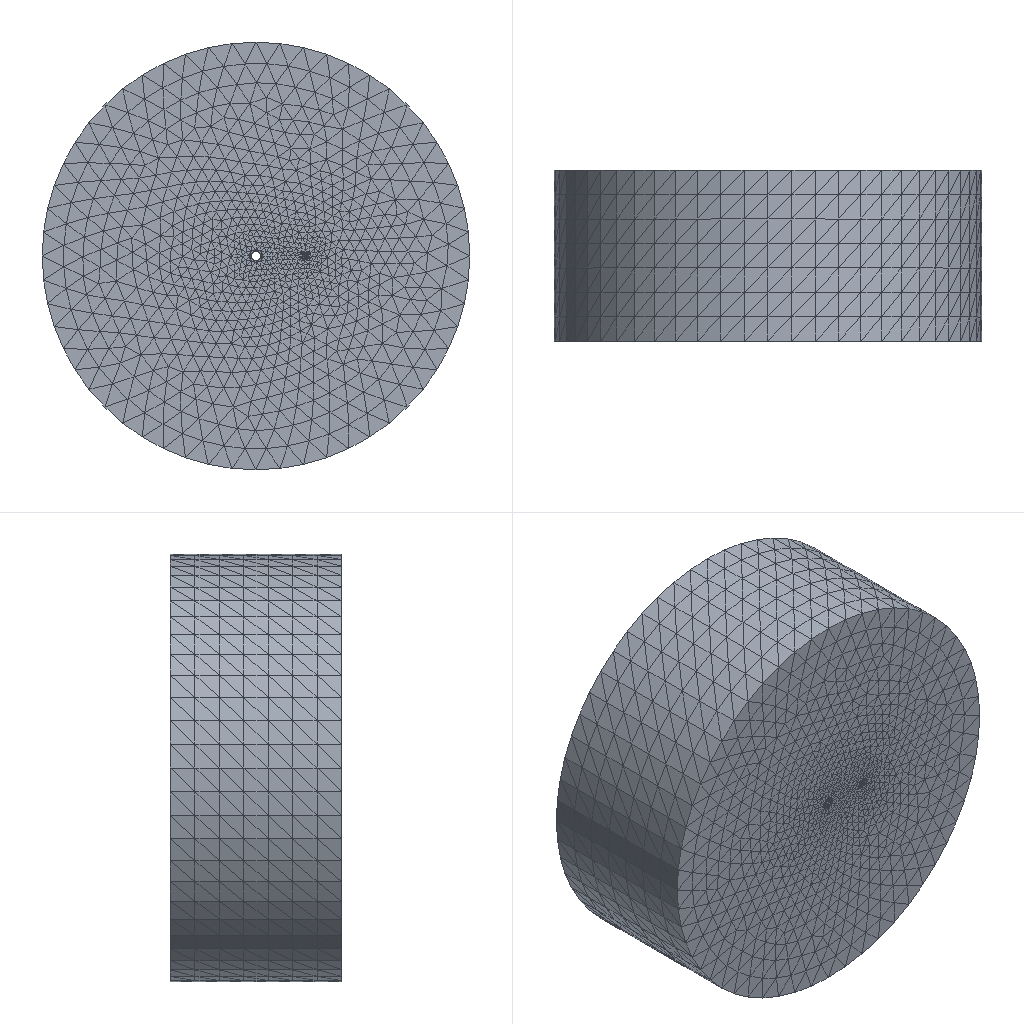Simulation study | abaqus
Set-up summary:
category,name,step,type,value,unit,region
solver,abaqus
solver,version,,,Abaqus/Standard 2020
units,not stated in the deck,,not stated
analysis,deck,,static,static
load_step,Step-1,Step-1,static
load_step,Step-2,Step-2,static
load_step,requested,,,2
mesh,nodes,,,19342
mesh,elements,,,80560
element_type,C3D4,,solid,80560
load,load commands in deck,,count,1
bc,support commands in deck,,count,1
material,CEMENT,,in results
material,SOIL,,in results
material,TUBE,,in results
check,setup vs results,,match,"per instance, exact: element labels, types and connectivity; labels of the nodes the elements use; coordinates of those nodes at SINGLE_PRECISION in 1 of 3 instance(s)"
Abaqus input file, long lists of numbers shortened:
*Heading
** Job name: Job-2 Model name: Model-1-Copy
** Generated by: Abaqus/CAE 2020
*Preprint, echo=NO, model=NO, history=NO, contact=NO
**
** PARTS
**
*Part, name=P21
*Node
      1,   1050.777,           0.,           0.
      2,   1258.624,           0.,           0.
** (8455 more lines like these left out)
*Element, type=C3D4
    1, 7574, 7583, 3286, 7573
    2, 7581, 3288, 3287, 3349
** (25295 more lines like these left out)
*Nset, nset=Set-1, generate
    1,  8457,     1
*Elset, elset=Set-1, generate
     1,  25297,      1
** Section: tube
*Solid Section, elset=Set-1, material=tube
,
*End Part
**
*Part, name=P22
*Node
      1,   1012.672,           0.,           0.
      2,   1296.729,           0.,           0.
** (1206 more lines like these left out)
*Element, type=C3D4
   1, 1188, 1190,  609, 1193
   2, 1188,    8, 1191,  610
** (3563 more lines like these left out)
*Nset, nset=Set-1, generate
    1,  1208,     1
*Elset, elset=Set-1, generate
    1,  3565,     1
*Nset, nset=Set-2, generate
    1,  1208,     1
*Elset, elset=Set-2, generate
    1,  3565,     1
** Section: cement
*Solid Section, elset=Set-2, material=cement
,
*End Part
**
*Part, name=P23
*Node
      1,           0.,           0.,        5000.
      2,           0.,           0.,       -5000.
** (9675 more lines like these left out)
*Element, type=C3D4
    1, 2201, 2202, 2203, 2204
    2, 2201, 2202, 2205, 2203
** (51696 more lines like these left out)
*Nset, nset=Set-1, generate
    1,  9677,     1
*Elset, elset=Set-1, generate
     1,  51698,      1
** Section: soil
*Solid Section, elset=Set-1, material=soil
,
*End Part
**
**
** ASSEMBLY
**
*Assembly, name=Assembly
**
*Instance, name=P21-1, part=P21
*End Instance
**
*Instance, name=P22-1, part=P22
*End Instance
**
*Instance, name=P23-1, part=P23
          0.,        4000.,           0.
          0.,        4000.,           0.,           1.,        4000., 6.12323426292584e-17,         180.
*End Instance
**
*Nset, nset=Set-1, instance=P21-1
   1,   2,   3,   4,   9,  10,  11,  12,  17,  18,  19,  20,  21,  22,  23,  24
  25,  26,  27,  28,  29,  30,  31,  32,  33,  34,  35,  36,  37,  38,  39,  40
** (4 more lines like these left out)
*Nset, nset=Set-1, instance=P22-1
   1,   2,   3,   4,   9,  10,  11,  12,  17,  18,  19,  20,  21,  22,  23,  24
  25,  26,  27,  28, 102, 103, 104, 105, 106, 107, 108, 109, 110, 111, 112, 113
** (1 more lines like these left out)
*Nset, nset=Set-1, instance=P23-1
    5,    6,    9,   10,   11,   12,   88,   89,   90,   91,   92,   93,  112,  113,  114,  115
  116,  117,  124,  125,  126,  127,  128,  129,  130,  131,  132,  133,  134,  135,  136,  137
** (53 more lines like these left out)
*Elset, elset=Set-1, instance=P21-1
   838,   844,   850,   902,   938,  1491,  6031, 10297, 10301, 10312, 10314, 10326, 10328, 10341, 10342, 10361
 10389, 10392, 10394, 10405, 10420, 10436, 10440, 10451, 10465, 10466, 10468, 10473, 10474, 10481, 10482, 10487
** (4 more lines like these left out)
*Elset, elset=Set-1, instance=P22-1
  149,  506, 1424, 1821, 1826, 1873, 1874, 1875, 1877, 1884, 1888, 1903, 1908, 1922, 1933, 1938
 1939, 1941, 2226, 2269, 2361, 2533, 2537, 2561, 2767, 2825, 2836, 2842, 2846, 2847, 2848, 3042
** (1 more lines like these left out)
*Elset, elset=Set-1, instance=P23-1
    15,   152,   213,   350,   508,   532,   550,   619,   665,   831,  1279,  1311,  1422,  1458,  1522,  1597
  1651,  1745,  1796,  1807,  1938,  2013,  2113,  2181,  2314,  2352,  2353,  2435,  2530,  2604,  2626,  2627
** (103 more lines like these left out)
*Nset, nset=Set-2, instance=P21-1, generate
    1,  8457,     1
*Nset, nset=Set-2, instance=P22-1, generate
    1,  1208,     1
*Nset, nset=Set-2, instance=P23-1, generate
    1,  9677,     1
*Elset, elset=Set-2, instance=P21-1, generate
     1,  25297,      1
*Elset, elset=Set-2, instance=P22-1, generate
    1,  3565,     1
*Elset, elset=Set-2, instance=P23-1, generate
     1,  51698,      1
*Nset, nset=Set-3, instance=P21-1, generate
    1,  8457,     1
*Nset, nset=Set-3, instance=P22-1, generate
    1,  1208,     1
*Nset, nset=Set-3, instance=P23-1, generate
    1,  9677,     1
*Elset, elset=Set-3, instance=P21-1, generate
     1,  25297,      1
*Elset, elset=Set-3, instance=P22-1, generate
    1,  3565,     1
*Elset, elset=Set-3, instance=P23-1, generate
     1,  51698,      1
*Nset, nset=Set-4, instance=P21-1, generate
    1,  8457,     1
*Nset, nset=Set-4, instance=P22-1, generate
    1,  1208,     1
*Nset, nset=Set-4, instance=P23-1, generate
    1,  9677,     1
*Elset, elset=Set-4, instance=P21-1, generate
     1,  25297,      1
*Elset, elset=Set-4, instance=P22-1, generate
    1,  3565,     1
*Elset, elset=Set-4, instance=P23-1, generate
     1,  51698,      1
*Elset, elset=_Surf-1_S3, internal, instance=P21-1
     2,     3,     8,    15,    31,    34,    47,    52,    72,    76,    84,    95,    96,   102,   110,   123
   124,   147,   149,   153,   177,   183,   185,   186,   189,   202,   206,   207,   217,   228,   235,   245
** (439 more lines like these left out)
*Elset, elset=_Surf-1_S4, internal, instance=P21-1
    29,    37,   119,   143,   154,   167,   325,   397,   465,   499,   565,   610,   652,   667,   673,   718
   773,   838,   844,   864,   913,   920,   938,   945,   955,   966,   992,  1009,  1011,  1015,  1066,  1087
** (22 more lines like these left out)
*Elset, elset=_Surf-1_S1, internal, instance=P21-1
   223,   420,   443,   459,   693,   785,   830,   866,  1608,  1623,  2301,  2526,  3215,  3218,  3593,  3598
  3692,  4192,  4402,  4443,  4547,  4582,  4586,  4798,  5314,  5372,  5657,  5929,  6073,  6639,  6643,  7053
** (13 more lines like these left out)
*Elset, elset=_Surf-1_S2, internal, instance=P21-1
    21,    54,   273,   331,   336,   367,   449,   491,   522,   543,   612,   653,   655,   658,  1065,  1111
  1139,  1180,  1261,  1290,  1705,  2255,  2774,  2778,  2863,  3034,  3327,  3662,  4244,  4304,  4344,  4485
** (16 more lines like these left out)
*Surface, type=ELEMENT, name=Surf-1
_Surf-1_S3, S3
_Surf-1_S4, S4
_Surf-1_S2, S2
_Surf-1_S1, S1
*Elset, elset=_Surf-2_S4, internal, instance=P21-1
    11,    13,    26,    29,    37,    38,    58,    59,    78,    88,    93,   112,   119,   122,   127,   143
   145,   154,   159,   167,   171,   174,   187,   190,   196,   199,   212,   243,   262,   285,   297,   300
** (158 more lines like these left out)
*Elset, elset=_Surf-2_S4, internal, instance=P22-1
    7,   12,   22,   26,   32,   54,   55,   59,   61,   75,   87,  104,  106,  125,  141,  142
  169,  170,  182,  189,  192,  194,  199,  203,  219,  226,  235,  241,  243,  258,  259,  288
** (23 more lines like these left out)
*Elset, elset=_Surf-2_S4, internal, instance=P23-1
   293,  1215,  1422,  1704,  2620,  2635,  2721,  2737,  2758,  2882,  2966,  3146,  3160,  3288,  3450,  3914
  4023,  4055,  4489,  4644,  4717,  4811,  4903,  5114,  5203,  5349,  5376,  5379,  5392,  5576,  5614,  5738
** (8 more lines like these left out)
*Elset, elset=_Surf-2_S2, internal, instance=P21-1
     1,     7,    12,    21,    23,    27,    35,    54,    56,    66,    67,    74,    77,    90,    94,    99
   105,   116,   125,   131,   134,   135,   140,   144,   156,   160,   161,   168,   178,   181,   184,   191
** (204 more lines like these left out)
*Elset, elset=_Surf-2_S2, internal, instance=P22-1
    1,    3,   14,   18,   23,   25,   36,   38,   39,   41,   45,   56,   66,   71,   73,   78
   79,   84,   90,   92,   93,   99,  100,  101,  107,  116,  117,  121,  122,  126,  129,  136
** (35 more lines like these left out)
*Elset, elset=_Surf-2_S2, internal, instance=P23-1
    15,   213,  1425,  2671,  2680,  2681,  2697,  2946,  3058,  3136,  3248,  3276,  3288,  3625,  3774,  3778
  3922,  4321,  4378,  4380,  4426,  4580,  4736,  4740,  4848,  4913,  5018,  5098,  5140,  5172,  5368,  5369
** (10 more lines like these left out)
*Elset, elset=_Surf-2_S1, internal, instance=P21-1
    17,    18,    19,    28,    42,    45,    46,    48,    57,    63,    71,    73,    79,    80,    82,    89
   100,   104,   111,   113,   117,   120,   136,   137,   150,   169,   173,   188,   193,   194,   197,   201
** (219 more lines like these left out)
*Elset, elset=_Surf-2_S1, internal, instance=P22-1
    2,    4,    6,    8,   10,   15,   16,   20,   21,   27,   28,   37,   43,   44,   51,   53
   63,   64,   69,   80,   86,   94,  102,  111,  130,  133,  148,  149,  156,  157,  162,  167
** (28 more lines like these left out)
*Elset, elset=_Surf-2_S1, internal, instance=P23-1
  2647,  2650,  2681,  2737,  4903,  5051,  5114,  5379,  5562,  5942,  5948,  5991,  6048,  6147,  6285,  6327
  6728,  6913,  7548,  7761,  7950,  7962,  8070,  8084,  8120,  8147,  8159,  8448,  8627,  8801,  8819,  8866
** (6 more lines like these left out)
*Elset, elset=_Surf-2_S3, internal, instance=P21-1
     2,     3,     8,    15,    31,    34,    47,    52,    72,    76,    84,    85,    95,    96,   102,   106
   108,   110,   123,   124,   141,   147,   149,   153,   175,   177,   183,   185,   186,   189,   202,   206
** (467 more lines like these left out)
*Elset, elset=_Surf-2_S3, internal, instance=P22-1
   13,   17,   24,   35,   47,   50,   97,   98,  108,  110,  113,  114,  115,  118,  128,  134
  137,  139,  144,  151,  153,  160,  161,  163,  174,  176,  196,  201,  207,  209,  212,  214
** (59 more lines like these left out)
*Elset, elset=_Surf-2_S3, internal, instance=P23-1
    27,    30,    53,    61,    90,   113,   114,   152,   174,   210,   218,   350,   398,   498,   502,   503
   508,   532,   550,   619,   665,   741,   831,   847,   928,  1058,  1143,  1209,  1243,  1279,  1311,  1319
** (245 more lines like these left out)
*Surface, type=ELEMENT, name=Surf-2
_Surf-2_S4, S4
_Surf-2_S2, S2
_Surf-2_S1, S1
_Surf-2_S3, S3
*Elset, elset=_Surf-3_S4, internal, instance=P21-1
    11,    13,    26,    29,    37,    38,    58,    59,    78,    88,    93,   112,   119,   122,   127,   143
   145,   154,   159,   167,   171,   174,   187,   190,   196,   199,   212,   243,   262,   285,   297,   300
** (158 more lines like these left out)
*Elset, elset=_Surf-3_S4, internal, instance=P22-1
    7,   12,   22,   26,   32,   54,   55,   59,   61,   75,   87,  104,  106,  125,  141,  142
  169,  170,  182,  189,  192,  194,  199,  203,  219,  226,  235,  241,  243,  258,  259,  288
** (23 more lines like these left out)
*Elset, elset=_Surf-3_S4, internal, instance=P23-1
   293,  1215,  1422,  1704,  2620,  2635,  2721,  2737,  2758,  2882,  2966,  3146,  3160,  3288,  3450,  3914
  4023,  4055,  4489,  4644,  4717,  4811,  4903,  5114,  5203,  5349,  5376,  5379,  5392,  5576,  5614,  5738
** (8 more lines like these left out)
*Elset, elset=_Surf-3_S2, internal, instance=P21-1
     1,     7,    12,    21,    23,    27,    35,    54,    56,    66,    67,    74,    77,    90,    94,    99
   105,   116,   125,   131,   134,   135,   140,   144,   156,   160,   161,   168,   178,   181,   184,   191
** (204 more lines like these left out)
*Elset, elset=_Surf-3_S2, internal, instance=P22-1
    1,    3,   14,   18,   23,   25,   36,   38,   39,   41,   45,   56,   66,   71,   73,   78
   79,   84,   90,   92,   93,   99,  100,  101,  107,  116,  117,  121,  122,  126,  129,  136
** (35 more lines like these left out)
*Elset, elset=_Surf-3_S2, internal, instance=P23-1
    15,   213,  1425,  2671,  2680,  2681,  2697,  2946,  3058,  3136,  3248,  3276,  3288,  3625,  3774,  3778
  3922,  4321,  4378,  4380,  4426,  4580,  4736,  4740,  4848,  4913,  5018,  5098,  5140,  5172,  5368,  5369
** (10 more lines like these left out)
*Elset, elset=_Surf-3_S1, internal, instance=P21-1
    17,    18,    19,    28,    42,    45,    46,    48,    57,    63,    71,    73,    79,    80,    82,    89
   100,   104,   111,   113,   117,   120,   136,   137,   150,   169,   173,   188,   193,   194,   197,   201
** (219 more lines like these left out)
*Elset, elset=_Surf-3_S1, internal, instance=P22-1
    2,    4,    6,    8,   10,   15,   16,   20,   21,   27,   28,   37,   43,   44,   51,   53
   63,   64,   69,   80,   86,   94,  102,  111,  130,  133,  148,  149,  156,  157,  162,  167
** (28 more lines like these left out)
*Elset, elset=_Surf-3_S1, internal, instance=P23-1
  2647,  2650,  2681,  2737,  4903,  5051,  5114,  5379,  5562,  5942,  5948,  5991,  6048,  6147,  6285,  6327
  6728,  6913,  7548,  7761,  7950,  7962,  8070,  8084,  8120,  8147,  8159,  8448,  8627,  8801,  8819,  8866
** (6 more lines like these left out)
*Elset, elset=_Surf-3_S3, internal, instance=P21-1
     2,     3,     8,    15,    31,    34,    47,    52,    72,    76,    84,    85,    95,    96,   102,   106
   108,   110,   123,   124,   141,   147,   149,   153,   175,   177,   183,   185,   186,   189,   202,   206
** (467 more lines like these left out)
*Elset, elset=_Surf-3_S3, internal, instance=P22-1
   13,   17,   24,   35,   47,   50,   97,   98,  108,  110,  113,  114,  115,  118,  128,  134
  137,  139,  144,  151,  153,  160,  161,  163,  174,  176,  196,  201,  207,  209,  212,  214
** (59 more lines like these left out)
*Elset, elset=_Surf-3_S3, internal, instance=P23-1
    27,    30,    53,    61,    90,   113,   114,   152,   174,   210,   218,   350,   398,   498,   502,   503
   508,   532,   550,   619,   665,   741,   831,   847,   928,  1058,  1143,  1209,  1243,  1279,  1311,  1319
** (245 more lines like these left out)
*Surface, type=ELEMENT, name=Surf-3
_Surf-3_S4, S4
_Surf-3_S2, S2
_Surf-3_S1, S1
_Surf-3_S3, S3
*Elset, elset=_m_Surf-4_S2, internal, instance=P21-1
     1,     7,    12,    23,    27,    35,    56,    66,    67,    74,    77,    90,    94,    99,   105,   116
   125,   131,   134,   135,   140,   144,   156,   160,   161,   168,   178,   181,   184,   191,   215,   216
** (137 more lines like these left out)
*Elset, elset=_m_Surf-4_S4, internal, instance=P21-1
    11,    13,    26,    38,    58,    78,    88,    93,   112,   122,   127,   145,   159,   171,   174,   187
   190,   196,   199,   212,   243,   262,   285,   297,   300,   316,   337,   344,   352,   378,   390,   404
** (90 more lines like these left out)
*Elset, elset=_m_Surf-4_S1, internal, instance=P21-1
    17,    18,    19,    28,    42,    45,    46,    48,    57,    63,    71,    73,    79,    80,    82,    89
   100,   104,   111,   113,   117,   120,   136,   137,   150,   169,   173,   188,   193,   194,   197,   201
** (148 more lines like these left out)
*Elset, elset=_m_Surf-4_S3, internal, instance=P21-1
    85,   106,   108,   141,   175,   211,   272,   345,   348,   368,   376,   417,   462,   471,   492,   498
   550,   551,   554,   564,   615,   640,   661,   682,   687,   735,   765,   803,   811,   889,   901,   915
** (17 more lines like these left out)
*Surface, type=ELEMENT, name=m_Surf-4
_m_Surf-4_S2, S2
_m_Surf-4_S4, S4
_m_Surf-4_S1, S1
_m_Surf-4_S3, S3
*Elset, elset=_m_Surf-6_S2, internal, instance=P22-1
    1,    3,   14,   18,   23,   25,   36,   38,   39,   41,   45,   66,   71,   73,   78,   79
   90,   93,   99,  100,  101,  107,  116,  117,  121,  122,  129,  136,  140,  147,  158,  159
** (19 more lines like these left out)
*Elset, elset=_m_Surf-6_S1, internal, instance=P22-1
    2,    6,    8,   10,   15,   16,   21,   27,   28,   37,   43,   44,   51,   53,   63,   64
   80,   94,  102,  111,  130,  133,  156,  157,  162,  167,  172,  173,  181,  197,  198,  215
** (15 more lines like these left out)
*Elset, elset=_m_Surf-6_S4, internal, instance=P22-1
    7,   12,   22,   26,   32,   54,   55,  104,  141,  142,  169,  170,  182,  199,  203,  226
  241,  259,  288,  304,  322,  323,  331,  355,  359,  385,  418,  425,  436,  443,  455,  462
** (8 more lines like these left out)
*Elset, elset=_m_Surf-6_S3, internal, instance=P22-1
   17,   50,  108,  114,  118,  134,  151,  153,  161,  176,  196,  209,  255,  264,  271,  289
  310,  551,  611,  734,  789,  805,  816,  827,  844,  918,  939,  943,  956,  975, 1002, 1009
** (2 more lines like these left out)
*Surface, type=ELEMENT, name=m_Surf-6
_m_Surf-6_S2, S2
_m_Surf-6_S1, S1
_m_Surf-6_S4, S4
_m_Surf-6_S3, S3
*Elset, elset=_s_Surf-4_S2, internal, instance=P22-1
   56,   84,  126,  263,  277,  460,  613,  614,  699,  748,  752,  904, 1102, 1108, 1251, 1252
 1274, 1283, 1333, 1337, 1338, 1339, 1373, 1429, 1443, 1447, 1450, 1451, 1467, 1553, 1584, 1673
** (4 more lines like these left out)
*Elset, elset=_s_Surf-4_S3, internal, instance=P22-1
   13,   24,   35,   47,   97,   98,  110,  113,  115,  128,  137,  139,  144,  160,  163,  174
  201,  207,  212,  214,  223,  228,  231,  233,  234,  238,  245,  267,  273,  274,  278,  281
** (53 more lines like these left out)
*Elset, elset=_s_Surf-4_S1, internal, instance=P22-1
    4,   20,   69,   86,  148,  149,  175,  188,  266,  369,  440,  478,  536,  722,  741,  757
  764,  857,  885,  898,  902,  909,  919,  992, 1077, 1093, 1117, 1120, 1302, 1380, 1445, 1448
** (4 more lines like these left out)
*Elset, elset=_s_Surf-4_S4, internal, instance=P22-1
   59,   61,   75,  106,  125,  189,  192,  194,  219,  235,  243,  258,  303,  334,  339,  379
  430,  451,  494,  578,  650,  681,  693,  697,  774,  779,  825,  850,  929,  953,  980, 1016
** (7 more lines like these left out)
*Surface, type=ELEMENT, name=s_Surf-4
_s_Surf-4_S2, S2
_s_Surf-4_S3, S3
_s_Surf-4_S4, S4
_s_Surf-4_S1, S1
*Elset, elset=_s_Surf-6_S3, internal, instance=P23-1
   113,  2445,  2454,  2467,  2494,  2580,  2618,  2650,  2656,  2661,  2675,  2682,  2686,  2687,  2711,  2727
  2747,  2753,  2754,  2855,  2863,  2924,  2936,  3141,  3147,  3270,  3293,  3338,  3399,  3442,  3477,  3544
** (29 more lines like these left out)
*Elset, elset=_s_Surf-6_S2, internal, instance=P23-1
  2680,  3058,  3136,  3276,  6688,  6694,  7196,  7224,  7651,  7764,  7931,  7936,  7968,  8152,  8158,  8593
  9731, 11220, 11245, 11502, 16204, 17280
*Elset, elset=_s_Surf-6_S4, internal, instance=P23-1
  3160,  3288,  3450,  4055,  6539,  7704,  7827,  7836,  7940,  7977,  8310,  8312, 11229, 11293, 12046, 12974
 19345, 22350, 22855, 24051, 25027, 35622, 36049
*Elset, elset=_s_Surf-6_S1, internal, instance=P23-1
  6913,  7548,  7950,  7962,  8070,  8120,  8147,  8159,  8448, 11391, 11736, 15689, 16349, 16350, 17668, 18025
 19647, 22604, 23977, 30785, 32849, 35625, 36410, 36685, 38378
*Surface, type=ELEMENT, name=s_Surf-6
_s_Surf-6_S3, S3
_s_Surf-6_S2, S2
_s_Surf-6_S4, S4
_s_Surf-6_S1, S1
** Constraint: Constraint-1
*Tie, name=Constraint-1, adjust=yes, position tolerance=1.
s_Surf-4, m_Surf-4
** Constraint: Constraint-2
*Tie, name=Constraint-2, adjust=yes, position tolerance=1.
s_Surf-6, m_Surf-6
*End Assembly
**
** MATERIALS
**
*Material, name=cement
*Density
 1.9e-09,
*Elastic
18000., 0.14
*Expansion
 1.05e-05,
*Material, name=soil
*Density
 2.3e-09,
*Elastic
17000., 0.2
*Expansion
 1.03e-05,
*Material, name=tube
*Density
 7.8e-09,
*Elastic
200000., 0.3
*Expansion
 1.22e-05,
**
** PHYSICAL CONSTANTS
**
*Physical Constants, absolute zero=-273., stefan boltzmann=5.67e-08
**
** BOUNDARY CONDITIONS
**
** Name: BC-1 Type: 对称/反对称/完全固定
*Boundary
Set-1, ENCASTRE
**
** PREDEFINED FIELDS
**
** Name: Predefined Field-1   Type: Temperature
*Initial Conditions, type=TEMPERATURE
Set-2, 50.
** ----------------------------------------------------------------
**
** STEP: Step-1
**
*Step, name=Step-1, nlgeom=YES, inc=10000
*Static, stabilize=0.0002, allsdtol=0.05, continue=NO
0.01, 1., 1e-05, 1.
**
** PREDEFINED FIELDS
**
** Name: Predefined Field-2   Type: Temperature
*Temperature, file=D:\___________\_____\_____._____________________
**
** OUTPUT REQUESTS
**
*Restart, write, frequency=0
**
** FIELD OUTPUT: F-Output-1
**
*Output, field, variable=PRESELECT
**
** HISTORY OUTPUT: H-Output-1
**
*Output, history, variable=PRESELECT
*End Step
** ----------------------------------------------------------------
**
** STEP: Step-2
**
*Step, name=Step-2, nlgeom=YES, inc=10000
*Static, stabilize=0.0002, allsdtol=0.05, continue=NO
0.01, 1., 1e-05, 1.
**
** PREDEFINED FIELDS
**
** Name: Predefined Field-1   Type: Temperature
*Temperature, op=NEW
Set-2, 50.
** Name: Predefined Field-2   Type: Temperature
*Temperature, op=NEW
** Name: Predefined Field-3   Type: Temperature
*Temperature, op=NEW, file=D:\___________\_____\_____._____________________
**
** OUTPUT REQUESTS
**
*Restart, write, frequency=0
**
** FIELD OUTPUT: F-Output-1
**
*Output, field
*Node Output
CF, RF, U
*Element Output, directions=YES
E, LE, MISES, PE, PEEQ, PEMAG, S
*Contact Output
CDISP, CSTRESS
**
** HISTORY OUTPUT: H-Output-1
**
*Output, history, variable=PRESELECT
*End Step
Results summary:
result,step,,completed,increments=11 time=1.0/1.0
result,step,,partial,increments=25 time=0.3639/1.0
result,analysis,,,static
result,last_loadstep,,,2
result,primary field,,,U
result,reaction total,,FX,182196.198,model units
result,reaction total,,FY,-1159266.678,model units
result,reaction total,,FZ,-2821.487,model units